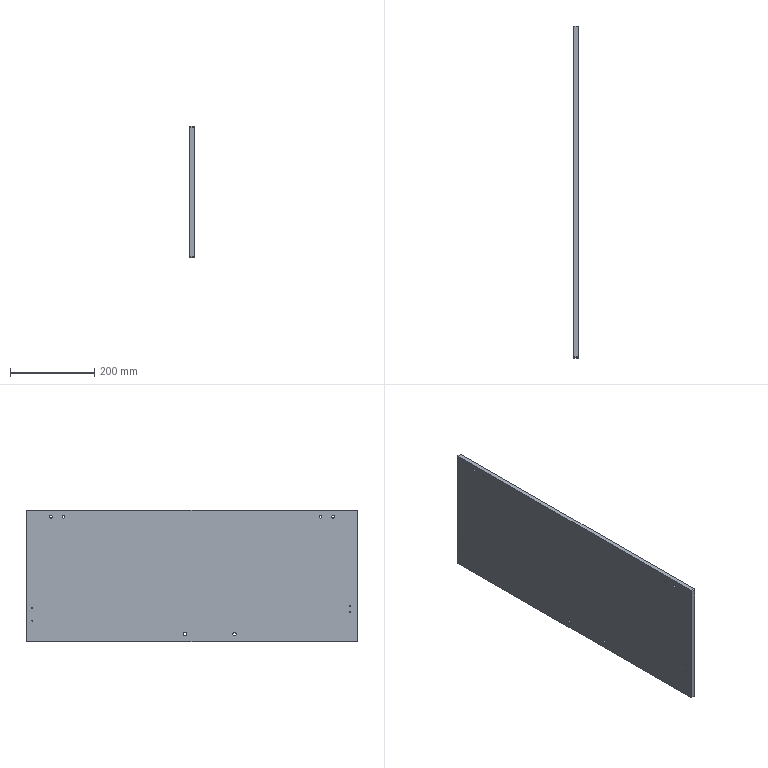Part | STEP file | 227H056118 DOOR L_Default | 1 solid | 30 faces | box 10 x 786 x 311 mm | volume 2441721 mm3 | cylinder 20 | plane 10 | commonest cylinder face diameters 2.5 x8 6.5 x8 8.5 x4